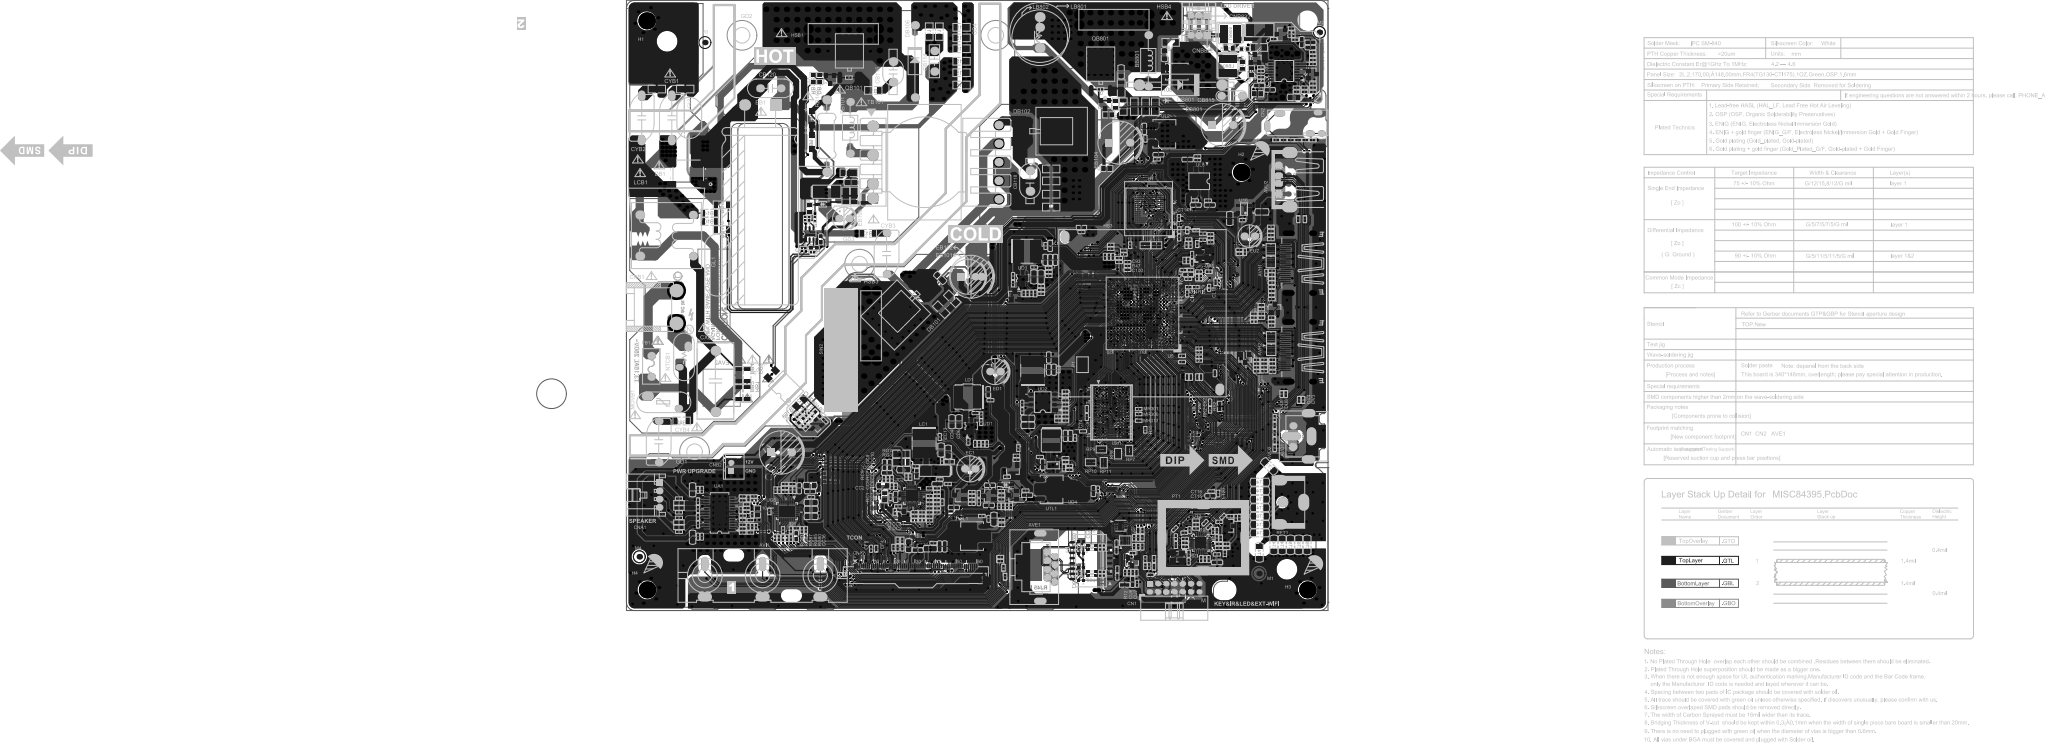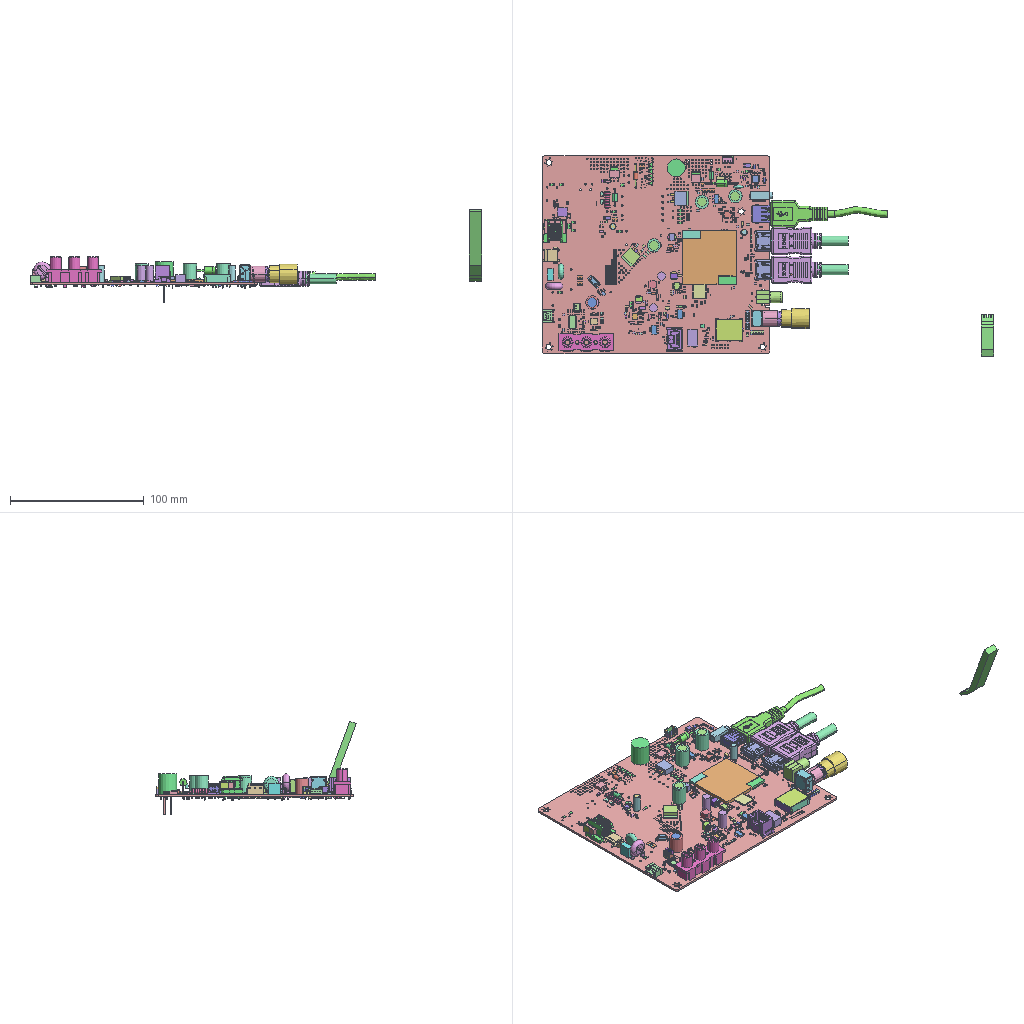Circuit board layout | Altium Designer | box 337.8 x 150 x 69.7 mm
Layer stack:
# Altium Designer layer stack of  (unit mm; dielectric type: 0 none, 1 core, 2 prepreg, 3 surface material)
index,name,kind,layer,copper_thickness_mm,dielectric_type,dielectric_thickness_mm,dielectric_material,dielectric_constant
0,TopPaste,other,,,,,,
1,TopOverlay,other,,,,,,
2,TopSolder,dielectric,,,3,0.0102,Solder Resist,3.5
3,TopLayer,copper,TopLayer,0.0356,,,,
4,Dielectric1,dielectric,,,1,1.5,FR-4,4.8
5,BottomLayer,copper,BottomLayer,0.0356,,,,
6,BottomSolder,dielectric,,,3,0.0102,Solder Resist,3.5
7,BottomOverlay,other,,,,,,
8,BottomPaste,other,,,,,,
# drill layer pairs: low layer,high layer
drill_pair,TopLayer,BottomLayer
Part placement, first 381 of 952 lines:
Designator,Comment,Layer,Footprint,Center-X(mm),Center-Y(mm),Rotation
RG02,NC/Thick film resistor,RES,1/16W,0ohm,¡À5%,0402,SMD,TopLayer,R0402,-79.121,21.946,360
RG01,NC/Thick film resistor,RES,1/16W,0ohm,¡À5%,0402,SMD,TopLayer,R0402,-83.896,22.911,180
LG02,0ohm-0402-¡À5%-1/16W,TopLayer,L0402,-79.121,20.803,360
LB805,Power inductor,2.2uH,¡À20%,2A,0.28¡Á1P,DR4.5¡Á3.2,SMD,PIO43-2R2MTP02,FH,TopLayer,L(4.5*3.5)-S,-23.673,139.903,0
CB815,NC/CK45-B3AD102KYPNX(TDK),TopLayer,CAP7.5*2.5-V-5,-23.393,124.79,360
AI_V,AI_GRIPPER_V,TopLayer,AI_GRIPPER_V,163.017,27.14,90
RB825,NC/Thick film resistor,RES,1/8W,0ohm,¡À5%,0805,SMD,TopLayer,R0805,-23.952,136.398,180
RB824,NC/Thick film resistor,RES,1/8W,0ohm,¡À5%,0805,SMD,TopLayer,R0805,-20.752,132.258,90
LB804,Power inductor,2.2uH,¡À20%,2A,0.28¡Á1P,DR4.5¡Á3.2,SMD,PIO43-2R2MTP02,FH,TopLayer,L(4.5*3.5)-S,-24.257,132.08,90
CT70,NC/4700pF-1206-X7R-¡À10%-1000V,TopLayer,C1206,-14.224,34.962,315
CT68,NC/4700pF-1206-X7R-¡À10%-1000V,TopLayer,C1206,-5.071,15.924,90
CT67,NC/4700pF-1206-X7R-¡À10%-1000V,TopLayer,C1206,-7.085,15.924,90
CT05,NC/33pF-0402-NPO-¡À5%-50V,TopLayer,C0402,-29.82,21.311,225
CT01,NC/33pF-0402-NPO-¡À5%-50V,TopLayer,C0402,-28.778,20.345,225
CM4,0.01uF-0402-X7R-¡À10%-50V,TopLayer,C0402,-43.021,8.661,180
CNB822,Connector socket,connect jack,3Pin,D2.0,L,SNAP,STEP,Fool-proofing,nature,L=2.8mm,DIP,CNJST,TopLayer,SIP3H/2.0D-3,-31.286,139.497,180
CB118,Ceramic capacitor,CAP CD,1KV,1000pF,¡À10%,Y5R,IK,5.0mm,DIP,TP,Walsin,TopLayer,CAP8.5*5-V-5,-72.212,104.165,270
CAUTION,CAUTION,BottomLayer,CAUTION,-612.141,-338.525,90
GL2,Silicone,0.5g,general,60,white,SLD-8854W,XY,TopLayer,Silica_gel-10,-612.141,-338.525,180
CB804,220pF-0402-NPO-¡À5%-50V,TopLayer,C0402,-16.275,129.335,360
RB116,NC/10ohm-1206-¡À5%-1/4W,TopLayer,R1206,-116.13,106.154,360
UB102,Regulator,IC Regulator,2.50V,0.4%,SOT-23,SMD,BR431M-A,Blue Rocket,TopLayer,SOT-23-RAK,-123.799,45.246,135
UB101,PWM controller,IC PWM Controller,65KHz,SOT-26,SMD,SR12 GL,Leadtrend,TopLayer,SOT-26,-125.615,91.342,180
TP-TDT,NC/,BottomLayer,TP-TDT,-153.187,110.735,90
TB101,Transformer,EQ2612,450uH,0.26¡Á2P,35Ts,H14.5MAX,SYEQ2612-T004,DIP,SQ,TopLayer,T/EQ2512*11,-95.096,108.725,0
RB821,NC/0R47ohm-1206-¡À1%-1/4W,TopLayer,R1206,-44.216,122.198,270
RB820,0R3ohm-1206-¡À5%-1/4W,TopLayer,R1206,-41.834,122.201,270
RB819,0R3ohm-1206-¡À5%-1/4W,TopLayer,R1206,-49.612,122.198,270
RB818,0R3ohm-1206-¡À5%-1/4W,TopLayer,R1206,-46.939,122.198,270
RB814,Thick film resistor,RES,1/8W,330Kohm,¡À1%,0805,SMD,TopLayer,R0805,-18.542,130.658,270
RB810,10ohm-1206-¡À5%-1/4W,TopLayer,R1206,-50.114,126.595,270
RB809,NC/10ohm-0805-¡À5%-1/8W,TopLayer,R0805,-53.134,120.193,180
RB808,10Kohm-0402-¡À5%-1/16W,TopLayer,R0402,-55.13,126.39,360
RB807,20ohm-0805-¡À5%-1/8W,TopLayer,R0805,-51.511,122.809,90
RB806,NC/30Kohm-0603-¡À5%-1/10W,TopLayer,R0603,-20.218,136.169,360
RB148,Metal oxide film resistor,RES MOF,2WS,0.36ohm,¡À5%,DIP,TP,Royalohm,TopLayer,R2-H-17.5,-121.463,115.081,90
RB142,2Mohm-1206-¡À5%-1/4W,TopLayer,R1206,-146.861,98.374,180
RB141,2Mohm-1206-¡À5%-1/4W,TopLayer,R1206,-149.867,96.368,180
RB140,51Kohm-0805-¡À1%-1/8W,TopLayer,R0805,-53.592,107.213,360
RB136,68ohm-1206-¡À5%-1/4W,TopLayer,R1206,-67.079,104.191,360
RB135,18Kohm-0402-¡À1%-1/16W,TopLayer,R0402,-127.051,45.034,45
RB134,4K7ohm-0402-¡À1%-1/16W,TopLayer,R0402,-126.314,44.298,45
RB133,10Kohm-0402-¡À1%-1/16W,TopLayer,R0402,-125.302,46.782,225
RB132,Thick film resistor,RES,1/16W,1.2Kohm,¡À1%,0402,SMD,TopLayer,R0402,-126.115,47.57,225
RB131,Thick film resistor,RES,1/10W,2Kohm,¡À1%,0603,SMD,TopLayer,R0603,-127.711,46.025,225
RB130,20ohm-1206-¡À5%-1/4W,TopLayer,R1206,-111.506,91.465,360
RB129,47ohm-1206-¡À5%-1/4W,TopLayer,R1206,-93.707,72.955,315
RB128,47ohm-1206-¡À5%-1/4W,TopLayer,R1206,-91.065,75.585,315
RB126,68ohm-1206-¡À5%-1/4W,TopLayer,R1206,-67.079,107.086,360
RB125,68ohm-1206-¡À5%-1/4W,TopLayer,R1206,-67.079,97.841,360
RB124,68ohm-1206-¡À5%-1/4W,TopLayer,R1206,-67.079,100.965,360
RB118,10ohm-1206-¡À5%-1/4W,TopLayer,R1206,-96.63,140.397,90
RB117,10ohm-1206-¡À5%-1/4W,TopLayer,R1206,-94.183,140.386,90
RB115,NC/4R7ohm-1206-¡À5%-1/4W,TopLayer,R1206,-114.837,100.563,270
RB114,4R7ohm-1206-¡À1%-1/4W,TopLayer,R1206,-116.84,100.568,270
RB109,10Kohm-0402-¡À1%-1/16W,TopLayer,R0402,-116.11,129.235,180
RB107,20ohm-0805-¡À5%-1/8W,TopLayer,R0805,-124.779,129.026,90
RB106,68ohm-0805-¡À5%-1/8W,TopLayer,R0805,-123.126,129.026,90
RB105,510ohm-0402-¡À1%-1/16W,TopLayer,R0402,-124.32,94.985,90
RB104,47Kohm-0402-¡À1%-1/16W,TopLayer,R0402,-124.86,86.901,180
RB103,Thick film resistor,RES,1/8W,6.8Kohm,¡À1%,0805,SMD,TopLayer,R0402,-126.706,95.017,270
RB102,330Kohm-1206-¡À5%-1/4W,TopLayer,R1206,-146.861,92.38,180
RB101,330Kohm-1206-¡À5%-1/4W,TopLayer,R1206,-149.857,94.361,360
RB3,1M2ohm-1206-¡À5%-1/4W,TopLayer,R1206,-140.757,57.05,90
RB1,1M2ohm-1206-¡À5%-1/4W,TopLayer,R1206,-140.757,52.681,90
QB801,MOSFET,NMOS,15A,100V,0.105ohm@ID=6A@VGS=10V,TO-252,PA110BDA,UNIKC,TopLayer,TO-252-GDS,-55.075,129.66,0
PWM_DIM,NC/TEST,BottomLayer,TP_BL,-2.515,124.028,270
PCB101,LTV-817S-TA-B(Lite-On),TopLayer,OC4-S-1,-131.342,53.854,45
ML1,NC/Latest Mylar sheet,TopLayer,Mylar,-612.141,-338.525,90
LB801,Differential-mode inductor,Inductor,DR12¡Á12,70uH,0.15¡Á12P,38.5Ts,H13.5MAX,SYDR1212-L070uA,DIP,EDL,TopLayer,L/LC2/15*14.5-V7.5,-69.853,140.166,90
GD4,NC/7.00¡Á8.35mm-nylon-white-WQM,TopLayer,Fixed,-80.5,139.5,0
GD3,NC/7.00¡Á8.35mm-nylon-white-WQM,TopLayer,Fixed,-113.5,84,0
GD2,NC/7.00¡Á8.35mm-nylon-white-WQM,TopLayer,Fixed,-142,139.5,0
GD1,NC/7.00¡Á8.35mm-nylon-white-WQM,TopLayer,Fixed,-153.5,38.5,0
EVA3,NC/7¡Á7¡Á3mm-C-4305 fire-retardant foam-black,BottomLayer,EVA(7*7*3),-612.141,-338.525,180
EVA2,NC/7¡Á7¡Á3mm-C-4305 fire-retardant foam-black,BottomLayer,EVA(7*7*3),-612.141,-338.525,180
EVA1,NC/7¡Á7¡Á3mm-C-4305 fire-retardant foam-black,BottomLayer,EVA(7*7*3),-612.141,-338.525,180
EB801,Aluminium electrolytic capacitor,CAP AL,63V,100uF,¡À20%,LD,PKLF,P,5.0mm,10¡Á12.5,DIP,TP,Koshin,TopLayer,EC(10*12.5)-V-5,-25.583,117.729,360
EB106,10uF-50V-¡À20%-5¡Á11-105¡æ-GH-taped reel-F=2.5(CapXon),TopLayer,EC(5*11)-V-2.5,-117.292,94.679,360
EB104,Aluminium electrolytic capacitor,CAP AL,35V,330uF,¡À20%,LD,PKZF,P,5.0mm,10¡Á12.5,DIP,TP,Koshin,TopLayer,EC(10*12.5)-V-5,-50.533,113.462,360
EB102,NC/270uF-16V-¡À20%-8¡Á11.5-105¡æ-PS-short pins-F=3.5(Capxon),TopLayer,EC(8*11)-V-3.5,-87.252,80.95,360
DB802,NC/M7(WEJ),TopLayer,DIODE-S-2,-16.586,140.741,180
DB801,NC/Schottky diode,DIO SBD S,3A,100V,DO-201AD,DIP,SR3100,YJ,TopLayer,D3-H-20,-35.793,127.483,360
DB111,Switching diode,DIO SW D1,215mA,85V,SOT-23,SMD,KAV70,KEXIN,TopLayer,SO-23,-120.624,128.818,360
DB106,Rectifier diode,DIO FRD S,1A,1000V,DO-41,DIP,FR107G,YJ,TopLayer,D1-H-17.5,-100.101,133.172,90
DB104,Rectifier diode,DIO SI S,1A,1000V,SMAF,SMD,M7F,YJ,TopLayer,DIODE-S-2,-121.529,101.557,180
DB102,Schottky diode,DIO SBD D1,10A,150V,TO-263,SMD,HBR10150SS,JLHW,TopLayer,D2PAK3,-69.501,116.244,180
DB101,Schottky diode,DIO SBD D1,10A,150V,TO-252,SMD,MBR10150GCT,PINGWEI,TopLayer,D2PAK3,-99.916,76.498,45
CYB4,NC/Y capacitor,CAP Y1,CD,470pF,400VAC,¡À20%,KS,10mm,Y5U,DIP,Walsin,TopLayer,CAP13*5-V-10-1,-162.179,40.923,270
CYB3,Y capacitor,CAP Y1,CD,470pF,400VAC,¡À20%,KS,10mm,Y5U,DIP,Walsin,TopLayer,CAP13*5-V-10-1,-106.959,86.567,270
CYB2,Y capacitor,CAP Y1,CD,470pF,400VAC,¡À20%,KS,10mm,Y5U,DIP,Walsin,TopLayer,CAP13*5-V-10-1,-166.294,119.478,90
CYB1,Y capacitor,CAP Y1,CD,470pF,400VAC,¡À20%,KS,10mm,Y5U,DIP,Walsin,TopLayer,CAP13*5-V-10-1,-159.004,119.478,90
CB809,220PF-0805-NPO-¡À10%-200V,TopLayer,C0805,-50.14,130.633,90
CB120,NC/Ceramic capacitor,CAP CD,1KV,4700pF,¡À20%,Y5U,K,5.0mm,DIP,TP,Walsin,TopLayer,CAP10*4.5-V-5,-135.117,126.644,360
CB117,1000pF-0805-NPO-¡À10%-200V,TopLayer,C0805,-93.977,80.642,315
CB116,Ceramic capacitor,CAP CD,2KV,100pF,¡À5%,SL,IK,5.0mm,DIP,TP,Walsin,TopLayer,CAP6.5*5-V-5-1,-105.385,130.621,90
CB114,Film capacitor,CAP PE,400V,4700pF,¡À10%,P,5.0mm,PC,DIP,TP,KEMET,TopLayer,CAP8*2.5-V-5,-95.377,133.212,270
CB113,NC/220PF-0805-NPO-¡À10%-200V,TopLayer,C0805,-115.595,103.792,180
CB111,Ceramic capacitor,CAP MC,50V,220pF,¡À5%,NPO,0603,SMD,TP,TopLayer,C0603,-124.625,87.993,180
CB110,NC/1000pF-0402-X7R-¡À10%-50V,TopLayer,C0402,-121.954,46.033,315
CB109,Ceramic capacitor,CAP MC,25V,0.22uF,¡À10%,X7R,0603,SMD,TP,TopLayer,C0603,-123.707,47.684,135
CB103,1000pF-0402-X7R-¡À10%-50V,TopLayer,C0402,-127.056,87.917,180
CB102,0.1uF-0603-X7R-¡À10%-50V,TopLayer,C0603,-122.898,90.02,270
CB101,100pF-0402-NPO-¡À5%-50V,TopLayer,C0402,-125.741,95.017,90
BL_ON,NC/TEST,BottomLayer,TP_BL,-5.69,123.85,360
BB801,Ferrite bead,BEAD,70ohm Min,¦Õ3.5¡Á6.0¡Á0.65mm,DIP,TP,RH3.5¡Á6¡Á0.8-T-LF,DL,TopLayer,LB/3.5*6*12.5,-43.551,133.299,270
BB101,Ferrite bead,BEAD,70ohm Min,¦Õ3.5¡Á6.0¡Á0.65mm,DIP,TP,RH3.5¡Á6¡Á0.8-T-LF,DL,TopLayer,LB/3.5*6*12.5,-115.799,117.086,270
ADIM,NC/TEST,BottomLayer,TP_BL,-7.899,140.183,270
CB125,NC/Ceramic capacitor,CAP MC,50V,0.022uF,¡À10%,X7R,0402,SMD,TP,TopLayer,C0402,-126.985,48.506,225
CNB832,NC/Connector socket,connect jack,3Pin,D2.0,D,L=2.8mm,DIP,AMA,TopLayer,SIP3/2.0D-CP,-31.293,144.272,180
Conformal Coating,NC/Conformal coating,25kg/Can,Peters,TopLayer,Conformal_Coating,-143.459,96.698,270
DB109,Rectifier diode,DIO FRD S,1.2A,800V,SOD-123FL,SMD,F1K,YJ,TopLayer,DIODE-S-14,-125.146,119.349,90
DB110,Rectifier diode,DIO FRD S,1.2A,800V,SOD-123FL,SMD,F1K,YJ,TopLayer,DIODE-S-14,-125.146,113.711,90
DB121,Switching diode,DIO SW S,200mA,250V,SOD-323,SMD,BAV21WS,BLUE ROCKET,TopLayer,DIODE-S-12,-122.453,98.527,360
DB807,NC/Schottky diode,DIO SBD S,3A,150V,TO-277,SMD,SBT03HL150T3TR,SL,TopLayer,DIODE-S-13,-37.385,130.689,270
DB809,NC/LBAV70LT1G(LRC),TopLayer,SO-23,-54.013,122.682,360
EVA4,NC/7¡Á7¡Á3mm-C-4305 fire-retardant foam-black,BottomLayer,EVA(7*7*3),-612.141,-338.525,90
HSB4,NC/Heat sink,17.5¡Á14.5¡Á0.5mm,copper sheet,matte tin plated,natural,four pins,WT,TopLayer,HS149-YZ,-51.867,143.281,180
LB802,NC/Differential-mode inductor,Inductor,DR12¡Á14,68uH,0.45,20Ts,H13.5MAX,SYDR1214-L068uA,DIP,Soldier,TopLayer,L(13.5*15.5)-V-5,-69.853,138.916,90
RB119,10ohm-1206-¡À5%-1/4W,TopLayer,R1206,-110.184,126.136,360
RB121,Thick film resistor,RES,1/8W,27Kohm,¡À1%,0805,SMD,TopLayer,R0805,-125.641,97.493,270
RB151,150Kohm-1206-¡À5%-1/4W,TopLayer,R1206,-88.789,136.246,360
RB152,150Kohm-1206-¡À5%-1/4W,TopLayer,R1206,-88.789,130.423,180
RB153,150Kohm-1206-¡À5%-1/4W,TopLayer,R1206,-88.789,127.441,180
RB154,150Kohm-1206-¡À5%-1/4W,TopLayer,R1206,-88.789,138.871,360
RB155,150Kohm-1206-¡À5%-1/4W,TopLayer,R1206,-88.789,141.437,360
RB156,150Kohm-1206-¡À5%-1/4W,TopLayer,R1206,-88.789,133.207,180
RB158,NC/Thick film resistor,RES,1/16W,51ohm,¡À1%,0402,SMD,TopLayer,R0402,-128.294,47.197,225
ZB801,NC/Zener diode,DIO ZEN,15V,300mW,SOT-23,SMD,BZX84C15,BLUE ROCKET,TopLayer,SO-23,-17.755,133.782,180
QB101,MOSFET,NMOS,5A,700V,0.8¦¸@ID=2.5A@VGS=10V,TO-252-2L,SVS5N70D,SL,TopLayer,TO-252-GDS,-115.969,132.874,360
CB802,220pF-0402-NPO-¡À5%-50V,TopLayer,C0402,-5.664,126.805,180
CB805,0.47uF-0805-X7R-¡À10%-50V,TopLayer,C0805,-8.186,124.443,360
CB806,1000pF-0402-X7R-¡À10%-50V,TopLayer,C0402,-16.276,130.833,360
CB807,220pF-0402-NPO-¡À5%-50V,TopLayer,C0402,-3.664,126.805,360
CB811,NC/1000pF-0402-X7R-¡À10%-50V,TopLayer,C0402,-7.601,126.801,180
CB813,0.1uF-0603-X7R-¡À10%-50V,TopLayer,C0603,-16.662,127.33,360
RB801,1Kohm-0402-¡À5%-1/16W,TopLayer,R0402,-3.664,125.789,180
RB802,10Kohm-0402-¡À5%-1/16W,TopLayer,R0402,-5.664,125.789,180
RB803,Thick film resistor,RES,1/16W,8.66Kohm,¡À1%,0402,SMD,TopLayer,R0402,-16.269,131.738,360
RB804,270ohm-0402-¡À5%-1/16W,TopLayer,R0402,-7.606,125.814,360
RB805,1Kohm-0402-¡À5%-1/16W,TopLayer,R0402,-16.275,128.422,360
RB812,NC/15Kohm-0402-¡À1%-1/16W,TopLayer,R0402,-3.675,133.506,360
RB816,2R2ohm-0805-¡À5%-1/8W,TopLayer,R0805,-17.081,125.324,180
RB822,Thick film resistor,RES,1/16W,15Kohm,¡À1%,0402,SMD,TopLayer,R0402,-3.675,134.471,360
RB827,510Kohm-0402-¡À1%-1/16W,TopLayer,R0402,-3.664,127.795,180
UB801,PWM controller,IC PWM Controller,200KHz,SOP-16,SMD,MP3398AGF-Z,MPS,TopLayer,TSSOP16/0.65-3,-10.607,130.908,180
CB803,0.1uF-0603-X7R-¡À10%-50V,TopLayer,C0603,-14.102,126.263,180
CB812,NC/1000pF-0402-X7R-¡À10%-50V,TopLayer,C0402,-3.675,132.537,360
DB806,Switching diode,DIO SW D1,215mA,85V,SOT-23,SMD,KAV70,KEXIN,TopLayer,SO-23,-3.784,129.997,90
CB810,220PF-0805-NPO-¡À10%-200V,TopLayer,C0805,-39.624,134.798,270
CB814,Ceramic capacitor,CAP MC,25V,1uF,¡À10%,X7R,0603,SMD,TP,TopLayer,C0603,-4.237,137.795,180
CB816,NC/Ceramic capacitor,CAP MC,25V,1uF,¡À10%,X7R,0603,SMD,TP,TopLayer,C0603,-4.237,136.525,180
QB525,General transistor,Dynatron,NPN,0.2A,40V,60-300,SOT-23,KMBT3904,KEXIN,TopLayer,SOT-23,-11.38,139.725,270
RB811,10ohm-1206-¡À5%-1/4W,TopLayer,R1206,-38.124,137.77,360
RB826,NC/10ohm-1206-¡À5%-1/4W,TopLayer,R1206,-16.739,136.55,180
RB830,Thick film resistor,RES,1/16W,3Kohm,¡À1%,0402,SMD,TopLayer,R0402,-7.976,138.43,180
RB832,Thick film resistor,RES,1/16W,30Kohm,¡À1%,0402,SMD,TopLayer,R0402,-13.157,138.582,360
RB833,Thick film resistor,RES,1/16W,2Kohm,¡À1%,0402,SMD,TopLayer,R0402,-8.382,139.758,270
RB834,Thick film resistor,RES,1/16W,2Kohm,¡À1%,0402,SMD,TopLayer,R0402,-8.839,141.148,360
RB837,Thick film resistor,RES,1/16W,12Kohm,¡À1%,0402,SMD,TopLayer,R0402,-3.702,135.407,360
EB1,Aluminium electrolytic capacitor,CAP AL,450V,82uF,¡À20%,SL,KL,BK,7.5mm,18¡Á35.5,DIP,CapXon,TopLayer,EC(18*41)-H-7.5-1,-137.601,122.617,360
EB101,Aluminium electrolytic capacitor,CAP AL,25V,470uF,¡À20%,LD,PKLH,P,5.0mm,10¡Á12.5,DIP,TP,Koshin,TopLayer,EC(10*12.5)-V-5,-86.502,80.95,360
FB1,Slow-blow fuse,FUSE T,P,3.15A,250VAC,8.4¡Á4.0¡Á7.2mm,DIP,TP,LS,TopLayer,FUSE8.5*4-V-5(T3.15AL_250V~),-163.998,59.207,90
CNB1,Connector socket,connect jack,2Pin,D7.92,L,SNAP,Fool-proofing,Nature,L=2.8mm,DIP,W7913-02RVA-S39SY,XYDT,TopLayer,CON2-H7.92,-157.988,73.609,360
CXB1,X capacitor,CAP X2,MP,280VAC,0.33uF,¡À10%,S,15mm,PC,DIP,JH,TopLayer,CAP18*8.5-V-15,-148.428,55.677,90
DB1,Bridge rectifier,DIO BRD,3A,800V,YBS,SMD,YBS3010A,YJ,TopLayer,B/YBS3010A,-155.016,105.893,270
GL1,Silicone,0.5g,general,60,white,SLD-8854W,XY,TopLayer,Silica_gel-15,-612.141,-338.525,360
LCB1,Common-mode choke,UU10.5,18mH MIN,0.35¡Á1P,80Ts,H14.5MAX,SYUU10.5-L002,DIP,CK,TopLayer,L/UU10.5/10*13-2,-160.272,90.928,90
MOVB1,Varistor,VARISTOR,128J,680V,4000A,S,7.5mm,10mm,DIP,Thinking,TopLayer,VR(13*5)-V-7.5,-161.052,50.497,180
NTCB1,SCK102R55AMBY502(short pins/Weiqin),TopLayer,NTC(10*5)-V5,-156.048,61.519,90
RB2,1M2ohm-1206-¡À5%-1/4W,TopLayer,R1206,-142.789,52.681,90
RB4,1M2ohm-1206-¡À5%-1/4W,TopLayer,R1206,-142.789,57.05,90
RB6,NC/0ohm-1206-PCB-D,TopLayer,R1206SC,-162.636,126.459,360
RB7,NC/0ohm-1206-PCB-D,TopLayer,R1206SC,-155.753,126.459,360
HSB3,NC/Heat sink,17.5¡Á14.5¡Á0.5mm,copper sheet,matte tin plated,natural,four pins,WT,TopLayer,HS149-YZ,-110.724,69.046,270
CB818,NC/1000pF-0402-X7R-¡À10%-50V,TopLayer,C0402,-9.322,139.758,90
CB819,NC/Ceramic capacitor,CAP MC,25V,1uF,¡À10%,X7R,0603,SMD,TP,TopLayer,C0603,-6.35,137.846,270
HSB1,NC/Heat sink,17.5¡Á14.5¡Á0.5mm,copper sheet,matte tin plated,natural,four pins,WT,TopLayer,HS149-YZ,-117.459,139.832,180
M3,MARK,TopLayer,MARK,-150.978,137.744,0
High Voltage,High Voltage,TopLayer,High_Voltage,-612.141,-338.525,360
RC28,Thick film resistor,RES,1/10W,22ohm,¡À5%,0603,SMD,TopLayer,R0603,-91.796,36.068,360
DV4,NC/TVS diode,DIO ESD,8pF,10V,0402,SMD,AZ5725-01F.R7GR,Amazing,TopLayer,DIODE-S0402,-7.01,51.054,90
DV3,NC/TVS diode,DIO ESD,8pF,10V,0402,SMD,AZ5725-01F.R7GR,Amazing,TopLayer,DIODE-S0402,-6.045,51.054,90
DA2,NC/AIES12U020R2-D,BottomLayer,DIODE-S0402,-34.798,81.61,270
DA1,NC/AIES12U020R2-D,TopLayer,DIODE-S0402,-28.88,82.169,180
CQC,CQC,TopLayer,CQC,-612.141,-338.525,270
CC35,Ceramic capacitor,CAP MC,50V,33pF,¡À5%,NPO,0402,SMD,TP,TopLayer,C0402,-93.523,36.246,90
CN2,Earphone jack,H,¦µ3.5,CH2.5,Black,switch,DIP,PJ-304L-EP,CS,TopLayer,PHONE-HD-54,-8.1,118.25,90
CT14,NC/0.1uF-0402-X5R-¡À20%-16V,TopLayer,C0402,-36.119,95.199,90
M6,MARK,BottomLayer,MARK,-2.083,140.208,180
M2,MARK,TopLayer,MARK,-2.083,140.208,0
COLD,COLD,TopLayer,COLD,-612.141,-338.525,360
H1,Location hole,TopLayer,ASSE4.0C-3,-165.177,143.186,180
HOT,HOT,TopLayer,HOT,-612.141,-338.525,360
MAC,MAC,BottomLayer,Barcode,-102.718,45.39,360
S/N2,Barcode,TopLayer,Barcode,-118.034,63.144,270
CL5,NC/10uF-0603-X5R-¡À20%-10V,TopLayer,C0603,-34.045,109.372,360
CL6,0.1uF-0402-X7R-¡À10%-16V,TopLayer,C0402,-31.658,110.134,180
CL9,0.1uF-0402-X7R-¡À10%-16V,TopLayer,C0402,-31.658,109.22,180
UL2,LC1117CLTR33,TopLayer,SOT-223,-39.682,115.595,270
RL1,NC/Thick film resistor,RES,1/16W,0ohm,¡À5%,0402,SMD,BottomLayer,R0402,-60.985,79.223,270
RL11,4K7ohm-0402-¡À5%-1/16W,BottomLayer,R0402,-53.797,81.426,90
RL4,NC/10Kohm-0402-¡À5%-1/16W,BottomLayer,R0402,-55.677,81.432,270
RL12,1Kohm-0402-¡À5%-1/16W,BottomLayer,R0402,-60.046,79.223,90
QL2,NC/General transistor,Dynatron,NPN,0.2A,40V,30-300,SOT-23,MMBT3904(f¡Ý350MHz),BLUE ROCKET,BottomLayer,SOT-23,-59.639,82.195,360
QL1,General transistor,Dynatron,NPN,0.2A,40V,30-300,SOT-23,MMBT3904(f¡Ý350MHz),BLUE ROCKET,BottomLayer,SOT-23,-57.862,78.359,90
DM3,TEST,BottomLayer,TP,-9.652,103.429,90
RF2,NC/1Mohm-0402-¡À5%-1/16W,TopLayer,R0402,-34.789,84.88,270
RF1,0ohm-0402-¡À5%-1/16W,TopLayer,R0402,-33.875,84.88,270
RU12,NC/4K7ohm-0402-¡À5%-1/16W,TopLayer,R0402,-13.839,90.068,180
RU9,10Kohm-0402-¡À5%-1/16W,TopLayer,R0402,-13.839,91.034,180
RU7,NC/4K7ohm-0402-¡À5%-1/16W,TopLayer,R0402,-13.839,93.066,180
RU3,10Kohm-0402-¡À5%-1/16W,TopLayer,R0402,-13.839,91.973,180
CU,NC/10uF-0805-X5R-¡À20%-16V,TopLayer,C0805,-23.796,95.071,270
CL10,NC/0.1uF-0402-X5R-¡À20%-16V,TopLayer,C0402,-21.484,87.452,180
RL6,100ohm-0402-¡À5%-1/16W,TopLayer,R0402,-21.484,86.512,360
UL5,LDO chip,IC LDO,1A,1.8&3.3V,12V,SOP-8,SMD,SA1118B-1833,SL,TopLayer,SOP8/1.27-3,-31.222,104.103,270
RT39,4K7ohm-0402-¡À5%-1/16W,TopLayer,R0402,-31.949,92.253,180
CL12,1uF-0402-X5R-¡À20%-6.3V,TopLayer,C0402,-32.263,99.441,360
CL11,NC/10uF-0603-X5R-¡À20%-6.3V,TopLayer,C0603,-32.06,98.349,360
CL8,1uF-0402-X5R-¡À20%-6.3V,TopLayer,C0402,-29.109,99.411,180
CL7,NC/10uF-0603-X5R-¡À20%-6.3V,TopLayer,C0603,-28.652,98.345,180
DP3,TEST,BottomLayer,TP,-9.627,105.613,90
D13,NC/TVS diode,DIO ESD,3pF,58V,0402,SMD,SDV1005H260C030YPTF,Sunlord,TopLayer,DIODE-S0402,-34.112,92.227,270
3V3_M,TEST,BottomLayer,TP,-34.362,95.707,180
H2,Location hole,TopLayer,ASSE4.0C-3,-21.076,106.436,180
1V8_M,TEST,BottomLayer,TP,-39.486,85.978,270
RP2,4*22ohm-0402-¡À5%-1/16W,TopLayer,RA0402,-41.56,88.579,270
R45,NC/0ohm-0402-PCB,BottomLayer,R0402SC,-41.079,83.534,270
R43,NC/0ohm-0402-PCB,BottomLayer,R0402SC,-42.849,76.748,270
R26,68ohm-0402-¡À5%-1/16W,BottomLayer,R0402,-37.024,77.184,180
R10,NC/10Kohm-0402-¡À5%-1/16W,BottomLayer,R0402,-41.017,97.352,270
R9,10Kohm-0402-¡À5%-1/16W,BottomLayer,R0402,-40.91,98.622,360
R4,NC/0ohm-0402-PCB,BottomLayer,R0402SC,-39.82,101.676,180
C63,0.1uF-0402-X7R-¡À10%-16V,BottomLayer,C0402,-40.834,80.004,180
C62,NC/1uF-0402-X5R-¡À20%-6.3V,BottomLayer,C0402,-40.834,78.759,180
C60,1uF-0402-X5R-¡À20%-6.3V,BottomLayer,C0402,-42.423,74.93,180
C59,0.1uF-0402-X7R-¡À10%-16V,BottomLayer,C0402,-42.469,83.16,180
C58,0.1uF-0402-X7R-¡À10%-16V,BottomLayer,C0402,-42.574,79.555,180
C57,0.1uF-0402-X7R-¡À10%-16V,BottomLayer,C0402,-42.574,80.441,180
C56,NC/10uF-0603-X5R-¡À20%-6.3V,BottomLayer,C0603,-42.228,87.664,180
C55,10uF-0603-X5R-¡À20%-6.3V,BottomLayer,C0603,-42.266,82.067,180
C23,0.047uF-0402-X7R-¡À10%-16V,BottomLayer,C0402,-37.888,76.269,360
C9,2.2uF-0402-X5R-¡À20%-6.3V,BottomLayer,C0402,-40.386,94.59,225
C4,0.1uF-0402-X5R-¡À20%-16V,BottomLayer,C0402,-44.282,95.066,360
C3,0.1uF-0402-X5R-¡À20%-16V,BottomLayer,C0402,-40.91,99.536,180
C2,1uF-0402-X5R-¡À20%-6.3V,BottomLayer,C0402,-42.456,97.453,270
C1,10uF-0603-X5R-¡À20%-6.3V,BottomLayer,C0603,-39.971,100.603,180
CVBS OUT,TEST,BottomLayer,TP,-39.818,76.447,90
C40,0.1uF-0402-X7R-¡À10%-16V,BottomLayer,C0402,-50.521,75.743,360
C108,NC/10uF-0603-X5R-¡À20%-6.3V,BottomLayer,C0603,-44.873,100.222,360
RP1,4*22ohm-0402-¡À5%-1/16W,TopLayer,RA0402,-44.273,88.579,270
R50,240ohm-0402-¡À1%-1/16W,BottomLayer,R0402,-46.99,77.655,90
R49,1Kohm-0402-¡À1%-1/16W,TopLayer,R0402,-49.496,87.293,360
R48,1Kohm-0402-¡À1%-1/16W,TopLayer,R0402,-52.654,88.671,360
R47,1Kohm-0402-¡À1%-1/16W,TopLayer,R0402,-48.597,83.578,180
R46,1Kohm-0402-¡À1%-1/16W,TopLayer,R0402,-52.654,87.732,180
R39,0ohm-0402-¡À5%-1/16W,BottomLayer,R0402,-43.751,76.168,270
R38,0ohm-0402-¡À5%-1/16W,BottomLayer,R0402,-44.64,76.168,270
R11,NC/10Kohm-0402-¡À5%-1/16W,BottomLayer,R0402,-46.473,98.215,360
R5,22ohm-0402-¡À5%-1/16W,TopLayer,R0402,-47.948,88.604,270
CL4,1uF-0402-X5R-¡À20%-6.3V,TopLayer,C0402,-44.247,114.427,270
CL3,NC/10uF-0603-X5R-¡À20%-6.3V,TopLayer,C0603,-44.501,116.815,90
CL2,0.1uF-0402-X5R-¡À20%-16V,TopLayer,C0402,-41.478,109.423,360
CL1,NC/10uF-0603-X5R-¡À20%-10V,TopLayer,C0603,-41.072,110.541,180
C101,1000pF-0402-X7R-¡À10%-50V,TopLayer,C0402,-49.495,86.353,360
C100,0.1uF-0402-X5R-¡À20%-16V,TopLayer,C0402,-48.597,82.626,180
C93,NC/0.01uF-0402-X7R-¡À10%-16V,TopLayer,C0402,-48.597,84.493,180
C86,0.01uF-0402-X7R-¡À10%-50V,TopLayer,C0402,-50.664,84.525,180
C66,0.1uF-0402-X7R-¡À10%-16V,BottomLayer,C0402,-45.736,74.873,360
C42,0.1uF-0402-X7R-¡À10%-16V,TopLayer,C0402,-52.148,85.803,270
C41,0.1uF-0402-X7R-¡À10%-16V,BottomLayer,C0402,-50.749,78.029,360
C39,NC/0.1uF-0402-X5R-¡À20%-16V,BottomLayer,C0402,-47.549,78.918,180
C38,NC/0.1uF-0402-X5R-¡À20%-16V,TopLayer,C0402,-54.053,85.803,270
C37,0.1uF-0402-X7R-¡À10%-16V,TopLayer,C0402,-53.087,85.803,270
C36,NC/Ceramic capacitor,CAP MC,6.3V,22uF,¡À20%,X5R,0603,SMD,TP,BottomLayer,C0603,-47.566,81.157,180
C35,Ceramic capacitor,CAP MC,6.3V,22uF,¡À20%,X5R,0603,SMD,TP,BottomLayer,C0603,-47.566,79.963,180
C34,Ceramic capacitor,CAP MC,6.3V,22uF,¡À20%,X5R,0603,SMD,TP,BottomLayer,C0603,-47.566,82.401,180
C33,10uF-0603-X5R-¡À20%-6.3V,BottomLayer,C0603,-50.8,79.604,360
C29,0.1uF-0402-X7R-¡À10%-16V,BottomLayer,C0402,-44.602,80.899,360
C28,0.1uF-0402-X7R-¡À10%-16V,BottomLayer,C0402,-44.602,79.984,360
C27,0.1uF-0402-X7R-¡À10%-16V,BottomLayer,C0402,-44.614,82.374,360
C26,NC/10uF-0603-X5R-¡À20%-6.3V,BottomLayer,C0603,-44.678,83.492,360
C25,10uF-0603-X5R-¡À20%-6.3V,BottomLayer,C0603,-44.729,78.918,360
C8,0.1uF-0402-X5R-¡À20%-16V,BottomLayer,C0402,-45.584,99.129,360
C7,0.1uF-0402-X5R-¡À20%-16V,BottomLayer,C0402,-46.498,97.301,360
C6,0.1uF-0402-X5R-¡À20%-16V,BottomLayer,C0402,-44.303,96.516,360
C5,1uF-0402-X5R-¡À20%-6.3V,BottomLayer,C0402,-43.374,99.13,180
R41,NC/0ohm-0402-PCB,BottomLayer,R0402SC,-48.831,74.974,360
R42,NC/0ohm-0402-PCB,BottomLayer,R0402SC,-47.028,75.939,270
RL5,100ohm-0402-¡À5%-1/16W,BottomLayer,R0402,-56.998,81.915,360
C126,NC/0.1uF-0402-X5R-¡À20%-16V,TopLayer,C0402,-50.664,85.49,180
CH2,1uF-0402-X5R-¡À20%-6.3V,TopLayer,C0402,-14.931,81.915,270
CT9,0.1uF-0402-X5R-¡À20%-16V,TopLayer,C0402,-34.281,88.639,270
CT1,33pF-0402-NPO-¡À5%-50V,TopLayer,C0402,-30.332,89.916,180
R3,0ohm-0402-¡À5%-1/16W,TopLayer,R0402,-31.744,80.765,270
CF5,Ceramic capacitor,CAP MC,50V,15pF,¡À5%,NPO,0402,SMD,TP,TopLayer,C0402,-32.935,84.372,270
RT40,4K7ohm-0402-¡À5%-1/16W,TopLayer,R0402,-28.448,89.306,360
RI12,12Kohm-0402-¡À1%-1/16W,BottomLayer,R0402,-34.078,80.207,180
RI11,10Kohm-0402-¡À5%-1/16W,BottomLayer,R0402,-30.192,78.835,270
RI9,12Kohm-0402-¡À1%-1/16W,BottomLayer,R0402,-32.122,78.81,270
RI7,10Kohm-0402-¡À5%-1/16W,BottomLayer,R0402,-31.208,78.81,270
RI5,75ohm-0402-¡À1%-1/16W,TopLayer,R0402,-32.046,78.429,180
RI4,33ohm-0402-¡À5%-1/16W,TopLayer,R0402,-33.748,78.429,360
R21,NC/1Kohm-0402-¡À5%-1/16W,TopLayer,R0402,-30.804,80.765,90
L3,GZ1005U121CTF(120ohm-500mA),TopLayer,L0402,-33.3,82.569,360
DH2,NC/22pF-0402-NPO-¡À5%-50V,TopLayer,DIODE-S0402,-13.611,80.487,180
DH1,NC/ULCE0505A015FR,TopLayer,DIODE-S0402,-13.631,81.453,180
D4,NC/SFI0402-240E-2R5PP-LF,TopLayer,DIODE-S0402,-31.287,82.188,360
CI9,1uF-0402-X5R-¡À20%-6.3V,TopLayer,C0402,-33.871,80.435,180
CI6,1uF-0402-X5R-¡À20%-6.3V,BottomLayer,C0402,-33.468,79.242,180
CI5,56pF-0402-NPO-¡À5%-50V,BottomLayer,C0402,-33.875,77.863,270
CI4,0.047uF-0402-X7R-¡À10%-16V,TopLayer,C0402,-34.129,76.879,90
CH3,NC/22pF-0402-NPO-¡À5%-50V,TopLayer,C0402,-13.631,82.405,180
CF6,Ceramic capacitor,CAP MC,50V,15pF,¡À5%,NPO,0402,SMD,TP,TopLayer,C0402,-32.935,86.252,90
C22,0.1uF-0402-X5R-¡À20%-16V,TopLayer,C0402,-35.072,82.569,180
C21,10uF-0603-X5R-¡À20%-6.3V,TopLayer,C0603,-33.852,81.502,180
CT2,0.1uF-0402-X5R-¡À20%-16V,TopLayer,C0402,-33.316,88.639,270
R33,4K7ohm-0402-¡À5%-1/16W,BottomLayer,R0402,-34.814,77.87,270
EU2,NC/Aluminium electrolytic capacitor,CAP AL,16V,100uF,¡À20%,RK,P,2.5mm,5¡Á11,DIP,TP,XL,TopLayer,EC(5*11)-V-2.5,-19.046,90.386,360
UH7,NC/TVS diode,DIO ESD,0.4pF,19V,DFN2510-10L,SMD,ESD5304D-10/TR,Willsemi,TopLayer,RCL0524P,-13.864,87.574,270
UH8,NC/TVS diode,DIO ESD,0.4pF,19V,DFN2510-10L,SMD,ESD5304D-10/TR,Willsemi,TopLayer,RCL0524P,-13.852,84.551,270
RT7,10Kohm-0402-¡À5%-1/16W,TopLayer,R0402,-36.043,92.278,270
CT5,33pF-0402-NPO-¡À5%-50V,TopLayer,C0402,-30.328,91.389,360
CT13,0.022uF-0402-X7R-¡À10%-16V,TopLayer,C0402,-36.059,90.468,90
CU1,10uF-0805-X5R-¡À20%-16V,TopLayer,C0805,-16.023,96.672,180
RT14,NC/?,TopLayer,R0402,-33.798,89.986,360
C103,NC/1uF-0402-X5R-¡À20%-16V,BottomLayer,C0402,-27.254,80.62,360
D14,NC/TVS diode,DIO ESD,3pF,58V,0402,SMD,SDV1005H260C030YPTF,Sunlord,TopLayer,DIODE-S0402,-31.699,88.919,270
U6,NC/SGM810-SXN3L,BottomLayer,SO-23-1,-28.219,82.702,90
U1,eMMC FLASH chip,IC EMMC FLASH,4GB,32Gb,MLC,FBGA153,SMD,KLM4G1FETE-B041,Samsung,TopLayer,BGA153/0.5-1,-43.481,97.448,180
S/N1,Barcode,BottomLayer,Barcode,-79.146,69.723,360
UD3,DC-DC chip,IC DC-DC,Syn,3A,18V,500kHz,SOT23-6,SMD,SY8113IADC,Silergy,TopLayer,TSOT23-6,-73.99,80.599,90
RH8,33ohm-0402-¡À5%-1/16W,TopLayer,R0402,-13.636,76.479,360
RH1,1Kohm-0402-¡À5%-1/16W,TopLayer,R0402,-13.636,77.47,360
RD27,NC/1Mohm-0402-¡À5%-1/16W,TopLayer,R0402,-67.673,81.175,360
RD26,100Kohm-0402-¡À5%-1/16W,TopLayer,R0402,-67.673,83.08,360
RD24,4K7ohm-0402-¡À5%-1/16W,TopLayer,R0402,-76.327,79.273,90
RD17,NC/?,TopLayer,R0402,-72.803,76.907,90
RD16,Thick film resistor,RES,1/16W,30Kohm,¡À1%,0402,SMD,TopLayer,R0402,-71.863,76.904,90
RD15,Thick film resistor,RES,1/16W,18.2Kohm,¡À1%,0402,SMD,TopLayer,R0402,-69.52,76.814,180
RD13,Thick film resistor,RES,1/16W,270Kohm,¡À1%,0402,SMD,TopLayer,R0402,-73.743,76.907,90
RD8,NC/,TopLayer,R0402,-69.518,78.687,360
QH1,General transistor,Dynatron,NPN,0.2A,40V,30-300,SOT-23,MMBT3904(f¡Ý350MHz),BLUE ROCKET,TopLayer,SOT-23,-12.975,73.305,180
LD3,Power inductor,2.2uH,¡À20%,3A,0.4¡Á1P,DR5.8¡Á4.5,SMD,DSB5845-2R2M-LF,BLDX,TopLayer,L(5.8*4.5)-S,-72.923,87.127,180
DH3,NC/22pF-0402-NPO-¡À5%-50V,TopLayer,DIODE-S0402,-13.624,79.509,180
CH4,NC/1000pF-0402-X7R-¡À10%-50V,TopLayer,C0402,-13.636,75.514,360
CH1,NC/1000pF-0402-X7R-¡À10%-50V,TopLayer,C0402,-13.624,78.46,360
CD45,10uF-0603-X5R-¡À20%-6.3V,TopLayer,C0603,-66.065,85.039,270
CD39,0.1uF-0402-X5R-¡À20%-16V,TopLayer,C0402,-67.673,82.115,360
CD21,NC/8pF-0402-NPO-¡À5%-50V,TopLayer,C0402,-70.949,76.904,270
CD20,NC/10uF-0603-X5R-¡À20%-6.3V,TopLayer,C0603,-67.335,88.422,90
CD19,10uF-0603-X5R-¡À20%-6.3V,TopLayer,C0603,-68.529,85.044,270
CD18,NC/10uF-0603-X5R-¡À20%-6.3V,TopLayer,C0603,-67.31,85.044,270
CD17,NC/0.1uF-0402-X5R-¡À20%-16V,TopLayer,C0402,-68.428,88.418,90
CD16,NC/NC/56pF-0402-NPO-¡À5%-50V,TopLayer,C0402,-69.517,77.748,360
CD15,NC/0.1uF-0402-X5R-¡À20%-16V,TopLayer,C0402,-71.196,83.21,360
CD13,NC/10uF-0805-X5R-¡À20%-16V,TopLayer,C0805,-69.52,80.904,270
CD14,10uF-0805-X5R-¡À20%-16V,TopLayer,C0805,-71.247,80.904,270
CD10,0.1uF-0402-X5R-¡À20%-16V,TopLayer,C0402,-76.327,81.111,90
3V3_STB,TEST,BottomLayer,TP,-42.062,107.34,90
U5,Customer-supplied main chip,IC Main Chip,SMD,MSD6A346ATT-8-XZ,COMPANY_A-QD,MTK,TopLayer,BGA406/0.8,-44.957,72.037,180
CD29,NC/0.1uF-0402-X5R-¡À20%-16V,TopLayer,C0402,-65.329,58.471,270
CD2,NC/10uF-0603-X5R-¡À20%-6.3V,TopLayer,C0603,-67.666,61.366,270
5V_STB,TEST,BottomLayer,TP,-82.249,60.35,90
RL8,4K7ohm-0402-¡À5%-1/16W,TopLayer,R0402,-20.138,86.944,270
QD1,MOSFET,NMOS,0.3A,60V,3.3ohm@ID=0.5A@VGS=10V,SOT-23,2N7002K1,BLUE ROCKET,TopLayer,SOT-23-7,-75.895,76.56,360
P1,NC/Conductive silicone,3¡Á2¡Á2.5mm,Black,Silicone Rubber,SMD,Joinset,TopLayer,Silica_gel(3*2*2.5),-59.487,59.614,90
CL13,NC/0.1uF-0402-X5R-¡À20%-16V,BottomLayer,C0402,-60.528,77.876,360
RL7,1Kohm-0402-¡À5%-1/16W,BottomLayer,R0402,-55.245,80.061,180
RL10,4K7ohm-0402-¡À5%-1/16W,BottomLayer,R0402,-54.737,81.432,90
RT2,100ohm-0402-¡À5%-1/16W,TopLayer,R0402,-28.473,91.24,180
RT4,100ohm-0402-¡À5%-1/16W,TopLayer,R0402,-28.467,90.322,180
U16,Current-limit switch,IC OCP,1.0A,5.5V,SOT23-5,SMD,APL3551CBI-TRG,ANPEC,TopLayer,SOT-23-5,-20.367,97.358,90
USB_5V,TEST,BottomLayer,TP,-9.652,101.016,90
Y1,Passive crystal oscillator,SPXO,24MHz,¡À10ppm,12pF,SMD3225-metal case,SMD,JWT,TopLayer,XTAL-S-3,-30.26,86.213,360
RS1,Ferrite bead,BEAD,120ohm,0603,2000mA,SMD,TP,HCB1608KF-121T20,TAI-TECH,TopLayer,R0603,-59.741,92.862,180
CS1,Ceramic capacitor,CAP MC,50V,22pF,¡À5%,NPO,0402,SMD,TP,TopLayer,C0402,-59.741,91.796,360
GND_JP2,NC,BottomLayer,GND,-31.877,80.924,180
GND_JP1,NC,BottomLayer,GND,-33.35,81.722,180
Pad and via stacks, first 74 of 302 lines:
# Altium Designer via and pad stacks of  (unit mm). Each distinct definition once, with the count of objects using it.
# via: kind,start_layer,end_layer,hole_mm,diameter_mm,mode(0 simple;1 top-mid-bottom;2 full stack),diameter_per_layer,count,example_net
# pad: kind,layer,hole_mm,hole_type(0 round;1 square;2 slot),plating,top_size,top_shape(1 round;2 rect;3 octagon;9 rounded rect),mid_size,bottom_size,mode,footprint,size_per_layer,count,example
pad,TopOverlay,0,0,plated,1.9x1.9,1,1.9x1.9,1.9x1.9,0,CAP7.5*2.5-V-5,,2,CB815.43
pad,TopOverlay,0,0,plated,1.6x1.6,1,1.6x1.6,1.6x1.6,0,SIP3H/2.0D-3,,2,CNB822.0
pad,TopOverlay,0,0,plated,1.6x1.6,2,1.6x1.6,1.6x1.6,0,SIP3H/2.0D-3,,1,CNB822.0
pad,TopOverlay,0,0,plated,2.1x2.1,1,2.1x2.1,2.1x2.1,0,CAP8.5*5-V-5,,2,CB118.0
pad,TopOverlay,0,0,plated,2.7x2.7,1,2.7x2.7,2.7x2.7,0,T/EQ2512*11,,4,TB101.2
pad,TopOverlay,0,0,plated,2x2,1,2x2,2x2,0,T/EQ2512*11,,5,TB101.12
pad,TopOverlay,0,0,plated,2.2x2.2,1,2.2x2.2,2.2x2.2,0,R2-H-17.5,,2,RB148.69
pad,TopOverlay,0,0,plated,2.4x2.4,1,2.4x2.4,2.4x2.4,0,L/LC2/15*14.5-V7.5,,2,LB801.1
pad,TopOverlay,0,0,plated,1.9x1.9,1,1.9x1.9,1.9x1.9,0,EC(10*12.5)-V-5,,3,EB801.1
pad,TopOverlay,0,0,plated,1.9x1.9,2,1.9x1.9,1.9x1.9,0,EC(10*12.5)-V-5,,3,EB801.1
pad,TopOverlay,0,0,unplated,1.8x1.8,1,1.8x1.8,1.8x1.8,0,EC(5*11)-V-2.5,,4,EB106.0
pad,TopOverlay,0,0,plated,1.8x1.8,2,1.8x1.8,1.8x1.8,0,EC(8*11)-V-3.5,,1,EB102.1
pad,TopOverlay,0,0,plated,1.8x1.8,1,1.8x1.8,1.8x1.8,0,EC(8*11)-V-3.5,,1,EB102.1
pad,TopOverlay,0,0,plated,2.6x2.6,1,2.6x2.6,2.6x2.6,0,D3-H-20,,2,DB801.0
pad,TopOverlay,0,0,plated,2x2,1,2x2,2x2,0,D1-H-17.5,,2,DB106.0
pad,TopOverlay,0,0,plated,1.9x1.9,1,1.9x1.9,1.9x1.9,0,CAP13*5-V-10-1,,4,CYB4.61
pad,TopOverlay,0,0,plated,1.9x2.55,1,1.9x2.55,1.9x2.55,0,CAP13*5-V-10-1,,4,CYB2.61
pad,TopOverlay,0,0,plated,1.9x1.9,1,1.9x1.9,1.9x1.9,0,CAP10*4.5-V-5,,2,CB120.42
pad,TopOverlay,0,0,plated,2.1x2.1,1,2.1x2.1,2.1x2.1,0,CAP6.5*5-V-5-1,,2,CB116.0
pad,TopOverlay,0,0,plated,2x2,1,2x2,2x2,0,CAP8*2.5-V-5,,2,CB114.1
pad,TopOverlay,0,0,plated,1.9x1.9,1,1.9x1.9,1.9x1.9,0,LB/3.5*6*12.5,,4,BB801.35
pad,TopOverlay,0,0,plated,1.4x1.4,2,1.4x1.4,1.4x1.4,0,SIP3/2.0D-CP,,1,CNB832.0
pad,TopOverlay,0,0,plated,1.4x1.4,1,1.4x1.4,1.4x1.4,0,SIP3/2.0D-CP,,2,CNB832.0
pad,TopOverlay,0,0,plated,2.1x2.1,1,2.1x2.1,2.1x2.1,0,L(13.5*15.5)-V-5,,2,LB802.3
pad,TopOverlay,0,0,plated,2.7x2.7,1,2.7x2.7,2.7x2.7,0,EC(18*41)-H-7.5-1,,1,EB1.1
pad,TopOverlay,0,0,plated,2.7x2.7,2,2.7x2.7,2.7x2.7,0,EC(18*41)-H-7.5-1,,1,EB1.1
pad,TopOverlay,0,0,plated,1.9x1.9,1,1.9x1.9,1.9x1.9,0,FUSE8.5*4-V-5(T3.15AL 250V~),,2,FB1.4
pad,TopOverlay,0,0,plated,3.2x3.2,1,3.2x3.2,3.2x3.2,0,CON2-H7.92,,2,CNB1.109
pad,TopOverlay,0,0,plated,2.4x2.4,1,2.4x2.4,2.4x2.4,0,CAP18*8.5-V-15,,2,CXB1.78
pad,TopOverlay,0,0,plated,2.2x2,1,2.2x2,2.2x2,0,L/UU10.5/10*13-2,,2,LCB1.4
pad,TopOverlay,0,0,plated,2.2x2.2,1,2.2x2.2,2.2x2.2,0,L/UU10.5/10*13-2,,2,LCB1.4
pad,TopOverlay,0,0,plated,2.1x1.8,1,2.1x1.8,2.1x1.8,0,VR(13*5)-V-7.5,,1,MOVB1.2
pad,TopOverlay,0,0,plated,2.2x3,1,2.2x3,2.2x3,0,VR(13*5)-V-7.5,,1,MOVB1.2
pad,TopOverlay,0,0,plated,2.4x1.9,1,2.4x1.9,2.4x1.9,0,NTC(10*5)-V5,,1,NTCB1.3
pad,TopOverlay,0,0,plated,1.6x2,1,1.6x2,1.6x2,0,NTC(10*5)-V5,,1,NTCB1.2
pad,TopOverlay,0,0,plated,1.9x1.9,1,1.9x1.9,1.9x1.9,0,EC(10*12)-V-5,,1,EA1.0
pad,TopOverlay,0,0,plated,1.9x1.9,2,1.9x1.9,1.9x1.9,0,EC(10*12)-V-5,,1,EA1.0
pad,TopOverlay,0,0,plated,1.8x1.8,1,1.8x1.8,1.8x1.8,0,EC(6.3*11)-V-2.5,,4,EC1.6
pad,TopOverlay,0,0,plated,0.8x0.28,1,0.8x0.28,0.8x0.28,0,DFN10/0.5-2,,1,DE2.6
pad,TopOverlay,0,0,plated,2x3.4,1,2x3.4,2x3.4,0,OPTICAL-HD-3,,2,AVO2.0
pad,TopOverlay,0,0,plated,1.778x1.778,1,1.778x1.778,1.778x1.778,0,OPTICAL-HD-3,,3,AVO2.0
pad,TopOverlay,0,0,plated,2.4x4.4,1,2.4x4.4,2.4x4.4,0,AV1-H-1,,1,AVO1.0
pad,TopOverlay,0,0,plated,2x4.6,1,2x4.6,2x4.6,0,AV1-H-1,,1,AVO1.0
pad,TopOverlay,0,0,plated,1.8x3.5,1,1.8x3.5,1.8x3.5,0,AV3-V14-1,,3,AVI1.0
pad,TopOverlay,0,0,plated,2.2x3.5,1,2.2x3.5,2.2x3.5,0,AV3-V14-1,,3,AVI1.0
pad,TopOverlay,0,0,plated,1.4x2.1,1,1.4x2.1,1.4x2.1,0,USB1-HD-2,,2,AVU2.2
pad,TopOverlay,0,0,plated,2.1x1.7,1,2.1x1.7,2.1x1.7,0,USB1-HD-2,,2,AVU2.0
pad,TopOverlay,0,0,plated,2.7x3.9,1,2.7x3.9,2.7x3.9,0,USB1-HD-2,,2,AVU2.0
pad,TopOverlay,0,0,unplated,2.7x4.1,1,2.7x4.1,2.7x4.1,0,ANT-IEC14.5-H-4,,1,RFT1.0
pad,TopOverlay,0,0,unplated,2.5x3.8,1,2.5x3.8,2.5x3.8,0,ANT-IEC14.5-H-4,,2,RFT1.0
pad,TopOverlay,0,0,plated,2.4x2.4,1,2.4x2.4,2.4x2.4,0,ANT-IEC14.5-H-4,,1,RFT1.0
pad,TopOverlay,0,0,plated,2.1x4.1,1,2.1x4.1,2.1x4.1,0,SHIELD(16*20*6),,4,PT1.0
pad,TopOverlay,0,0,plated,1.6x1.6,2,1.6x1.6,1.6x1.6,0,SIP4H/2.0D-6,,1,CNA1.0
pad,TopOverlay,0,0,plated,1.6x1.6,1,1.6x1.6,1.6x1.6,0,SIP4H/2.0D-6,,3,CNA1.0
pad,TopOverlay,0,0,plated,2.9x2.2,1,2.9x2.2,2.9x2.2,0,HS(40*40*2.3)-1,,2,HS3.2
pad,TopOverlay,0,0,plated,1.3x1.3,2,1.3x1.3,1.3x1.3,0,SIP2/2.0D-1,,1,CNB2.0
pad,TopOverlay,0,0,plated,1.3x1.3,1,1.3x1.3,1.3x1.3,0,SIP2/2.0D-1,,1,CNB2.0
pad,TopOverlay,0,0,plated,1.5x2.8,1,1.5x2.8,1.5x2.8,0,PHONE-HD-54,,2,CN2.0
pad,TopOverlay,0,0,plated,1.5x2.3,1,1.5x2.3,1.5x2.3,0,PHONE-HD-54,,1,CN2.0
pad,TopOverlay,0,0,plated,1.5x2,1,1.5x2,1.5x2,0,PHONE-HD-54,,1,CN2.0
pad,TopOverlay,0,0,plated,1.5x2.2,1,1.5x2.2,1.5x2.2,0,PHONE-HD-54,,1,CN2.0
pad,TopOverlay,0,0,plated,1.45x1.45,1,1.45x1.45,1.45x1.45,0,RJ45-VD-16,,8,AVE1.0
pad,TopOverlay,0,0,plated,3.1x1.6,1,3.1x1.6,3.1x1.6,0,RJ45-VD-16,,2,AVE1.0
pad,TopOverlay,0,0,plated,1.3x1.3,1,1.3x1.3,1.3x1.3,0,SIP2*7H/2.0DM-8,,13,CN1.0
pad,TopOverlay,0,0,plated,1.3x1.3,2,1.3x1.3,1.3x1.3,0,SIP2*7H/2.0DM-8,,1,CN1.0
pad,TopLayer,0,0,plated,0.5x0.45,2,0.5x0.45,0.5x0.45,0,R0402,,352,RG02.1
pad,TopLayer,0,0,plated,0.55x0.45,2,0.55x0.45,0.55x0.45,0,L0402,,18,LG02.1
pad,TopLayer,0,0,plated,4.3x1.8,2,4.3x1.8,4.3x1.8,0,L(4.5*3.5)-S,,6,LB805.1
pad,TopLayer,0,0,plated,1.4x1.8,2,1.4x1.8,1.4x1.8,0,FFC60H/0.5S-13,,2,CN12.62
pad,TopLayer,0,0,plated,0.3x1.1,1,0.3x1.1,0.3x1.1,0,FFC60H/0.5S-13,,59,CN12.50
pad,TopLayer,0,0,plated,0.3x1.1,2,0.3x1.1,0.3x1.1,0,FFC60H/0.5S-13,,1,CN12.1
Copper pours:
name,layer,net,type(0 solid;1 hatched;2 none)
5mil,BottomLayer,GND,0
5,BottomLayer,GND,0
5mil,BottomLayer,D_QB801,0
5mil,BottomLayer,GND,0
5mil,BottomLayer,D_QB101,0
5mil,BottomLayer,NetDB106_K,0
5,BottomLayer,GND,0
12,BottomLayer,GND,0
12,BottomLayer,RFGND,0
5mil,TopLayer,D_QB801,0
5mil,TopLayer,VBL,0
5mil,TopLayer,GND,0
5mil,TopLayer,D_QB101,0
5mil,TopLayer,VBRIDGE,0
5mil,TopLayer,NetCB114_1,0
5mil,TopLayer,NetDB106_K,0
5mil,TopLayer,SGND,0
5mil,TopLayer,NetCB118_2,0
5mil,TopLayer,L,0
5mil,TopLayer,N,0
5mil,TopLayer,GND,0
5mil,TopLayer,SGND,0
5,TopLayer,GND,0
5mil,TopLayer,GND,0
5,TopLayer,GND,0
5,TopLayer,GND,0
5,TopLayer,GND,0
5,TopLayer,GND,0
12,TopLayer,GND,0
12,TopLayer,RFGND,0
Design rules, without the lines most boards share, first 18 of 33 lines:
# Altium Designer design rules of  (exported by Altium Designer, unit mm)
# columns: name | kind | enabled | priority | scope1 | scope2 | descriptor | typed fields (field=value)
3.9mil for Minimum | 0 | enabled | 44 | Not ((IsTrack Or IsArc) And (Layer = 'KeepOutLayer')) | Not (IsPad or ((IsTrack Or IsArc) And (Layer = 'KeepOutLayer'))) | Clearance Constraint (Gap=3.9mil) (Not ((IsTrack Or IsArc) And (Layer = 'KeepOutLayer'))),(Not (IsPad or ((IsTrack Or IsArc) And (Layer = 'KeepOutLayer')))) | gap=0.0991
MS348T | 22 | enabled | 1 | InComponentClass('MS348T') | All | Room MS348T (Bounding Region = (21968.391mil, 15802.49mil, 22695.391mil, 16528.49mil) (InComponentClass('MS348T')) |
NetAntennae | 56 | enabled | 1 | Not (HasFootprint('ANT-7') or HasFootprint('ANT-BLUECORE')) | All | Net Antennae (Tolerance=40mil) (Not (HasFootprint('ANT-7') or HasFootprint('ANT-BLUECORE'))) |
Hole2Hole | 52 | disabled | 1 | All | All | Hole To Hole Clearance (Gap=18mil) (Disabled)(All),(All) | gap=0.4572
DiffPairsRouting | 51 | enabled | 4 | All | All | Differential Pairs Uncoupled Length using the Gap Constraints (Min=10mil) (Max=10mil) (Prefered=10mil)  and Width Constraints (Min=15mil) (Max=15mil) (Prefered=15mil) (All) |
TestPointUsage | 44 | enabled | 1 | All | All | Fabrication Testpoint Usage (Valid =One Required, Allow multiple per net=No) (All) |
Testpoint | 43 | enabled | 1 | All | All | Fabrication Testpoint Style (Under Component=Yes) (All) |
HoleSize_VIA | 42 | disabled | 1 | ISVIA | All | Hole Size Constraint (Min=7.874mil) (Max=23.622mil) (Disabled)(ISVIA) |
PermittedLayers | 26 | enabled | 1 | All | All | Permitted Layers - (Top Layer, Bottom Layer) (All) |
SMDToCorner | 23 | disabled | 1 | All | All | SMD To Corner (Distance=4mil) (Disabled)(All) |
MinimumAnnularRing | 19 | enabled | 1 | All | All | Minimum Annular Ring (Minimum=3.937mil) (All) |
ViasUnderSMD | 17 | enabled | 1 | All | All | Vias Under SMD Constraint (Allowed=Not Allowed) (All) |
PasteMaskExpansion | 14 | enabled | 1 | All | All | Paste Mask Expansion (Expansion =0mil) (All) | expansion=0
0.25_0.1 | 11 | disabled | 6 | All | All | Routing Via (MinHoleWidth=3.937mil) (MaxHoleWidth=3.937mil) (PreferredHoleWidth=3.937mil) (MinWidth=9.842mil) (MaxWidth=9.842mil) (PreferedWidth=9.842mil) (Disabled)(All) | via_min_hole=0.1 via_max_hole=0.1 via_preferred_diameter=0.25 via_preferred_hole=0.1
0.4_0.2 | 11 | disabled | 5 | All | All | Routing Via (MinHoleWidth=7.874mil) (MaxHoleWidth=7.874mil) (PreferredHoleWidth=7.874mil) (MinWidth=15.748mil) (MaxWidth=15.748mil) (PreferedWidth=15.748mil) (Disabled)(All) | via_min_hole=0.2 via_max_hole=0.2 via_preferred_diameter=0.4 via_preferred_hole=0.2
0.45_0.25 | 11 | disabled | 4 | All | All | Routing Via (MinHoleWidth=9.842mil) (MaxHoleWidth=9.842mil) (PreferredHoleWidth=9.842mil) (MinWidth=17.716mil) (MaxWidth=17.716mil) (PreferedWidth=17.716mil) (Disabled)(All) | via_min_hole=0.25 via_max_hole=0.25 via_preferred_diameter=0.45 via_preferred_hole=0.25